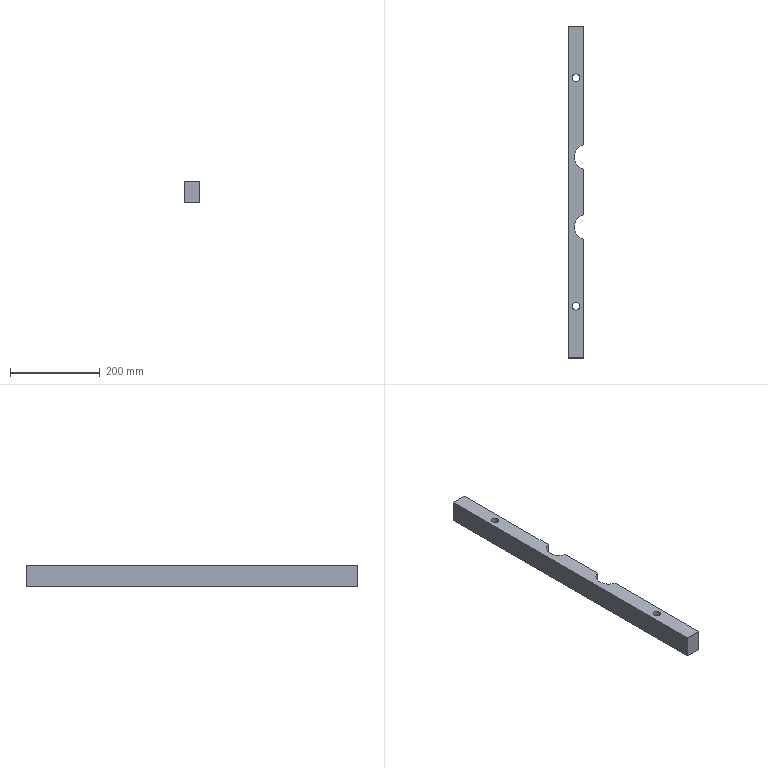Part | NX | features solid 2 | 1 solid | 12 faces | box 35 x 740 x 49 mm | volume 1163226 mm3 | plane 8 | cylinder 4 | commonest cylinder face diameters 17 x2 57 x2
STEP:
#1=CARTESIAN_POINT('',(868.,-370.,153.));
#2=VERTEX_POINT('',#1);
#3=CARTESIAN_POINT('',(868.,-370.,202.));
#4=VERTEX_POINT('',#3);
#5=CARTESIAN_POINT('',(868.,-370.,148.));
#6=DIRECTION('',(0.,0.,1.));
#7=VECTOR('',#6,1000.);
#8=LINE('',#5,#7);
#9=EDGE_CURVE('',#2,#4,#8,.T.);
#10=ORIENTED_EDGE('',*,*,#9,.F.);
#11=CARTESIAN_POINT('',(868.,-105.495,153.));
#12=VERTEX_POINT('',#11);
#13=CARTESIAN_POINT('',(868.,0.,153.));
#14=DIRECTION('',(0.,1.,0.));
#15=VECTOR('',#14,1000.);
#16=LINE('',#13,#15);
#17=EDGE_CURVE('',#2,#12,#16,.T.);
#18=ORIENTED_EDGE('',*,*,#17,.T.);
#19=CARTESIAN_POINT('',(868.,-105.495,202.));
#20=VERTEX_POINT('',#19);
#21=CARTESIAN_POINT('',(868.,-105.495,308.));
#22=DIRECTION('',(0.,0.,-1.));
#23=VECTOR('',#22,1000.);
#24=LINE('',#21,#23);
#25=EDGE_CURVE('',#12,#20,#24,.F.);
#26=ORIENTED_EDGE('',*,*,#25,.T.);
#27=CARTESIAN_POINT('',(868.,0.,202.));
#28=DIRECTION('',(0.,-1.,0.));
#29=VECTOR('',#28,1000.);
#30=LINE('',#27,#29);
#31=EDGE_CURVE('',#20,#4,#30,.T.);
#32=ORIENTED_EDGE('',*,*,#31,.T.);
#33=EDGE_LOOP('',(#10,#18,#26,#32));
#34=FACE_BOUND('',#33,.T.);
#35=CARTESIAN_POINT('',(868.,0.,148.));
#36=DIRECTION('',(1.,0.,0.));
#37=DIRECTION('',(0.,0.,-1.));
#38=AXIS2_PLACEMENT_3D('',#35,#36,#37);
#39=PLANE('',#38);
#40=ADVANCED_FACE('',(#34),#39,.T.);
#41=CARTESIAN_POINT('',(868.,-50.505,202.));
#42=VERTEX_POINT('',#41);
#43=CARTESIAN_POINT('',(868.,-50.505,153.));
#44=VERTEX_POINT('',#43);
#45=CARTESIAN_POINT('',(868.,-50.505,308.));
#46=DIRECTION('',(0.,0.,-1.));
#47=VECTOR('',#46,1000.);
#48=LINE('',#45,#47);
#49=EDGE_CURVE('',#42,#44,#48,.T.);
#50=ORIENTED_EDGE('',*,*,#49,.T.);
#51=CARTESIAN_POINT('',(868.,50.505,153.));
#52=VERTEX_POINT('',#51);
#53=CARTESIAN_POINT('',(868.,0.,153.));
#54=DIRECTION('',(0.,1.,0.));
#55=VECTOR('',#54,1000.);
#56=LINE('',#53,#55);
#57=EDGE_CURVE('',#44,#52,#56,.T.);
#58=ORIENTED_EDGE('',*,*,#57,.T.);
#59=CARTESIAN_POINT('',(868.,50.505,202.));
#60=VERTEX_POINT('',#59);
#61=CARTESIAN_POINT('',(868.,50.505,308.));
#62=DIRECTION('',(0.,0.,-1.));
#63=VECTOR('',#62,1000.);
#64=LINE('',#61,#63);
#65=EDGE_CURVE('',#52,#60,#64,.F.);
#66=ORIENTED_EDGE('',*,*,#65,.T.);
#67=CARTESIAN_POINT('',(868.,0.,202.));
#68=DIRECTION('',(0.,-1.,0.));
#69=VECTOR('',#68,1000.);
#70=LINE('',#67,#69);
#71=EDGE_CURVE('',#60,#42,#70,.T.);
#72=ORIENTED_EDGE('',*,*,#71,.T.);
#73=EDGE_LOOP('',(#50,#58,#66,#72));
#74=FACE_BOUND('',#73,.T.);
#75=CARTESIAN_POINT('',(868.,0.,148.));
#76=DIRECTION('',(1.,0.,0.));
#77=DIRECTION('',(0.,0.,-1.));
#78=AXIS2_PLACEMENT_3D('',#75,#76,#77);
#79=PLANE('',#78);
#80=ADVANCED_FACE('',(#74),#79,.T.);
#81=CARTESIAN_POINT('',(868.,105.495,202.));
#82=VERTEX_POINT('',#81);
#83=CARTESIAN_POINT('',(868.,105.495,153.));
#84=VERTEX_POINT('',#83);
#85=CARTESIAN_POINT('',(868.,105.495,308.));
#86=DIRECTION('',(0.,0.,-1.));
#87=VECTOR('',#86,1000.);
#88=LINE('',#85,#87);
#89=EDGE_CURVE('',#82,#84,#88,.T.);
#90=ORIENTED_EDGE('',*,*,#89,.T.);
#91=CARTESIAN_POINT('',(868.,370.,153.));
#92=VERTEX_POINT('',#91);
#93=CARTESIAN_POINT('',(868.,0.,153.));
#94=DIRECTION('',(0.,1.,0.));
#95=VECTOR('',#94,1000.);
#96=LINE('',#93,#95);
#97=EDGE_CURVE('',#84,#92,#96,.T.);
#98=ORIENTED_EDGE('',*,*,#97,.T.);
#99=CARTESIAN_POINT('',(868.,370.,202.));
#100=VERTEX_POINT('',#99);
#101=CARTESIAN_POINT('',(868.,370.,148.));
#102=DIRECTION('',(0.,0.,1.));
#103=VECTOR('',#102,1000.);
#104=LINE('',#101,#103);
#105=EDGE_CURVE('',#92,#100,#104,.T.);
#106=ORIENTED_EDGE('',*,*,#105,.T.);
#107=CARTESIAN_POINT('',(868.,0.,202.));
#108=DIRECTION('',(0.,-1.,0.));
#109=VECTOR('',#108,1000.);
#110=LINE('',#107,#109);
#111=EDGE_CURVE('',#100,#82,#110,.T.);
#112=ORIENTED_EDGE('',*,*,#111,.T.);
#113=EDGE_LOOP('',(#90,#98,#106,#112));
#114=FACE_BOUND('',#113,.T.);
#115=CARTESIAN_POINT('',(868.,0.,148.));
#116=DIRECTION('',(1.,0.,0.));
#117=DIRECTION('',(0.,0.,-1.));
#118=AXIS2_PLACEMENT_3D('',#115,#116,#117);
#119=PLANE('',#118);
#120=ADVANCED_FACE('',(#114),#119,.T.);
#121=CARTESIAN_POINT('',(842.,-255.,202.));
#122=VERTEX_POINT('',#121);
#123=CARTESIAN_POINT('',(850.5,-255.,202.));
#124=DIRECTION('',(0.,0.,1.));
#125=DIRECTION('',(-1.,0.,0.));
#126=AXIS2_PLACEMENT_3D('',#123,#124,#125);
#127=CIRCLE('',#126,8.5);
#128=EDGE_CURVE('',#122,#122,#127,.F.);
#129=ORIENTED_EDGE('',*,*,#128,.F.);
#130=EDGE_LOOP('',(#129));
#131=FACE_BOUND('',#130,.T.);
#132=CARTESIAN_POINT('',(842.,-255.,153.));
#133=VERTEX_POINT('',#132);
#134=CARTESIAN_POINT('',(850.5,-255.,153.));
#135=DIRECTION('',(0.,0.,-1.));
#136=DIRECTION('',(-1.,0.,0.));
#137=AXIS2_PLACEMENT_3D('',#134,#135,#136);
#138=CIRCLE('',#137,8.5);
#139=EDGE_CURVE('',#133,#133,#138,.F.);
#140=ORIENTED_EDGE('',*,*,#139,.F.);
#141=EDGE_LOOP('',(#140));
#142=FACE_BOUND('',#141,.T.);
#143=CARTESIAN_POINT('',(850.5,-255.,202.));
#144=DIRECTION('',(0.,0.,-1.));
#145=DIRECTION('',(-1.,0.,0.));
#146=AXIS2_PLACEMENT_3D('',#143,#144,#145);
#147=CYLINDRICAL_SURFACE('',#146,8.5);
#148=ADVANCED_FACE('',(#131,#142),#147,.F.);
#149=CARTESIAN_POINT('',(833.,370.,153.));
#150=VERTEX_POINT('',#149);
#151=CARTESIAN_POINT('',(833.,370.,202.));
#152=VERTEX_POINT('',#151);
#153=CARTESIAN_POINT('',(833.,370.,148.));
#154=DIRECTION('',(0.,0.,1.));
#155=VECTOR('',#154,1000.);
#156=LINE('',#153,#155);
#157=EDGE_CURVE('',#150,#152,#156,.T.);
#158=ORIENTED_EDGE('',*,*,#157,.F.);
#159=CARTESIAN_POINT('',(833.,-370.,153.));
#160=VERTEX_POINT('',#159);
#161=CARTESIAN_POINT('',(833.,0.,153.));
#162=DIRECTION('',(0.,-1.,0.));
#163=VECTOR('',#162,1000.);
#164=LINE('',#161,#163);
#165=EDGE_CURVE('',#150,#160,#164,.T.);
#166=ORIENTED_EDGE('',*,*,#165,.T.);
#167=CARTESIAN_POINT('',(833.,-370.,202.));
#168=VERTEX_POINT('',#167);
#169=CARTESIAN_POINT('',(833.,-370.,148.));
#170=DIRECTION('',(0.,0.,1.));
#171=VECTOR('',#170,1000.);
#172=LINE('',#169,#171);
#173=EDGE_CURVE('',#160,#168,#172,.T.);
#174=ORIENTED_EDGE('',*,*,#173,.T.);
#175=CARTESIAN_POINT('',(833.,0.,202.));
#176=DIRECTION('',(0.,1.,0.));
#177=VECTOR('',#176,1000.);
#178=LINE('',#175,#177);
#179=EDGE_CURVE('',#168,#152,#178,.T.);
#180=ORIENTED_EDGE('',*,*,#179,.T.);
#181=EDGE_LOOP('',(#158,#166,#174,#180));
#182=FACE_BOUND('',#181,.T.);
#183=CARTESIAN_POINT('',(833.,0.,148.));
#184=DIRECTION('',(-1.,0.,0.));
#185=DIRECTION('',(0.,0.,1.));
#186=AXIS2_PLACEMENT_3D('',#183,#184,#185);
#187=PLANE('',#186);
#188=ADVANCED_FACE('',(#182),#187,.T.);
#189=ORIENTED_EDGE('',*,*,#105,.F.);
#190=CARTESIAN_POINT('',(850.5,370.,153.));
#191=DIRECTION('',(-1.,0.,0.));
#192=VECTOR('',#191,1000.);
#193=LINE('',#190,#192);
#194=EDGE_CURVE('',#92,#150,#193,.T.);
#195=ORIENTED_EDGE('',*,*,#194,.T.);
#196=ORIENTED_EDGE('',*,*,#157,.T.);
#197=CARTESIAN_POINT('',(850.5,370.,202.));
#198=DIRECTION('',(1.,0.,0.));
#199=VECTOR('',#198,1000.);
#200=LINE('',#197,#199);
#201=EDGE_CURVE('',#152,#100,#200,.T.);
#202=ORIENTED_EDGE('',*,*,#201,.T.);
#203=EDGE_LOOP('',(#189,#195,#196,#202));
#204=FACE_BOUND('',#203,.T.);
#205=CARTESIAN_POINT('',(850.5,370.,148.));
#206=DIRECTION('',(0.,1.,0.));
#207=DIRECTION('',(0.,0.,1.));
#208=AXIS2_PLACEMENT_3D('',#205,#206,#207);
#209=PLANE('',#208);
#210=ADVANCED_FACE('',(#204),#209,.T.);
#211=ORIENTED_EDGE('',*,*,#173,.F.);
#212=CARTESIAN_POINT('',(850.5,-370.,153.));
#213=DIRECTION('',(1.,0.,0.));
#214=VECTOR('',#213,1000.);
#215=LINE('',#212,#214);
#216=EDGE_CURVE('',#160,#2,#215,.T.);
#217=ORIENTED_EDGE('',*,*,#216,.T.);
#218=ORIENTED_EDGE('',*,*,#9,.T.);
#219=CARTESIAN_POINT('',(850.5,-370.,202.));
#220=DIRECTION('',(-1.,0.,0.));
#221=VECTOR('',#220,1000.);
#222=LINE('',#219,#221);
#223=EDGE_CURVE('',#4,#168,#222,.T.);
#224=ORIENTED_EDGE('',*,*,#223,.T.);
#225=EDGE_LOOP('',(#211,#217,#218,#224));
#226=FACE_BOUND('',#225,.T.);
#227=CARTESIAN_POINT('',(850.5,-370.,148.));
#228=DIRECTION('',(0.,-1.,0.));
#229=DIRECTION('',(0.,0.,-1.));
#230=AXIS2_PLACEMENT_3D('',#227,#228,#229);
#231=PLANE('',#230);
#232=ADVANCED_FACE('',(#226),#231,.T.);
#233=CARTESIAN_POINT('',(842.,255.,202.));
#234=VERTEX_POINT('',#233);
#235=CARTESIAN_POINT('',(850.5,255.,202.));
#236=DIRECTION('',(0.,0.,-1.));
#237=DIRECTION('',(-1.,0.,0.));
#238=AXIS2_PLACEMENT_3D('',#235,#236,#237);
#239=CIRCLE('',#238,8.5);
#240=EDGE_CURVE('',#234,#234,#239,.T.);
#241=ORIENTED_EDGE('',*,*,#240,.F.);
#242=EDGE_LOOP('',(#241));
#243=FACE_BOUND('',#242,.T.);
#244=CARTESIAN_POINT('',(842.,255.,153.));
#245=VERTEX_POINT('',#244);
#246=CARTESIAN_POINT('',(850.5,255.,153.));
#247=DIRECTION('',(0.,0.,-1.));
#248=DIRECTION('',(-1.,0.,0.));
#249=AXIS2_PLACEMENT_3D('',#246,#247,#248);
#250=CIRCLE('',#249,8.5);
#251=EDGE_CURVE('',#245,#245,#250,.F.);
#252=ORIENTED_EDGE('',*,*,#251,.F.);
#253=EDGE_LOOP('',(#252));
#254=FACE_BOUND('',#253,.T.);
#255=CARTESIAN_POINT('',(850.5,255.,202.));
#256=DIRECTION('',(0.,0.,-1.));
#257=DIRECTION('',(-1.,0.,0.));
#258=AXIS2_PLACEMENT_3D('',#255,#256,#257);
#259=CYLINDRICAL_SURFACE('',#258,8.5);
#260=ADVANCED_FACE('',(#243,#254),#259,.F.);
#261=ORIENTED_EDGE('',*,*,#65,.F.);
#262=CARTESIAN_POINT('',(875.5,78.,153.));
#263=DIRECTION('',(0.,0.,-1.));
#264=DIRECTION('',(-1.,0.,0.));
#265=AXIS2_PLACEMENT_3D('',#262,#263,#264);
#266=CIRCLE('',#265,28.5);
#267=EDGE_CURVE('',#52,#84,#266,.T.);
#268=ORIENTED_EDGE('',*,*,#267,.T.);
#269=ORIENTED_EDGE('',*,*,#89,.F.);
#270=CARTESIAN_POINT('',(875.5,78.,202.));
#271=DIRECTION('',(0.,0.,1.));
#272=DIRECTION('',(1.,0.,0.));
#273=AXIS2_PLACEMENT_3D('',#270,#271,#272);
#274=CIRCLE('',#273,28.5);
#275=EDGE_CURVE('',#60,#82,#274,.F.);
#276=ORIENTED_EDGE('',*,*,#275,.F.);
#277=EDGE_LOOP('',(#261,#268,#269,#276));
#278=FACE_BOUND('',#277,.T.);
#279=CARTESIAN_POINT('',(875.5,78.,308.));
#280=DIRECTION('',(0.,0.,-1.));
#281=DIRECTION('',(-1.,0.,0.));
#282=AXIS2_PLACEMENT_3D('',#279,#280,#281);
#283=CYLINDRICAL_SURFACE('',#282,28.5);
#284=ADVANCED_FACE('',(#278),#283,.F.);
#285=ORIENTED_EDGE('',*,*,#25,.F.);
#286=CARTESIAN_POINT('',(875.5,-78.,153.));
#287=DIRECTION('',(0.,0.,-1.));
#288=DIRECTION('',(-1.,0.,0.));
#289=AXIS2_PLACEMENT_3D('',#286,#287,#288);
#290=CIRCLE('',#289,28.5);
#291=EDGE_CURVE('',#12,#44,#290,.T.);
#292=ORIENTED_EDGE('',*,*,#291,.T.);
#293=ORIENTED_EDGE('',*,*,#49,.F.);
#294=CARTESIAN_POINT('',(875.5,-78.,202.));
#295=DIRECTION('',(0.,0.,1.));
#296=DIRECTION('',(1.,0.,0.));
#297=AXIS2_PLACEMENT_3D('',#294,#295,#296);
#298=CIRCLE('',#297,28.5);
#299=EDGE_CURVE('',#20,#42,#298,.F.);
#300=ORIENTED_EDGE('',*,*,#299,.F.);
#301=EDGE_LOOP('',(#285,#292,#293,#300));
#302=FACE_BOUND('',#301,.T.);
#303=CARTESIAN_POINT('',(875.5,-78.,308.));
#304=DIRECTION('',(0.,0.,-1.));
#305=DIRECTION('',(-1.,0.,0.));
#306=AXIS2_PLACEMENT_3D('',#303,#304,#305);
#307=CYLINDRICAL_SURFACE('',#306,28.5);
#308=ADVANCED_FACE('',(#302),#307,.F.);
#309=ORIENTED_EDGE('',*,*,#128,.T.);
#310=EDGE_LOOP('',(#309));
#311=FACE_BOUND('',#310,.T.);
#312=ORIENTED_EDGE('',*,*,#240,.T.);
#313=EDGE_LOOP('',(#312));
#314=FACE_BOUND('',#313,.T.);
#315=ORIENTED_EDGE('',*,*,#31,.F.);
#316=ORIENTED_EDGE('',*,*,#299,.T.);
#317=ORIENTED_EDGE('',*,*,#71,.F.);
#318=ORIENTED_EDGE('',*,*,#275,.T.);
#319=ORIENTED_EDGE('',*,*,#111,.F.);
#320=ORIENTED_EDGE('',*,*,#201,.F.);
#321=ORIENTED_EDGE('',*,*,#179,.F.);
#322=ORIENTED_EDGE('',*,*,#223,.F.);
#323=EDGE_LOOP('',(#315,#316,#317,#318,#319,#320,#321,#322));
#324=FACE_BOUND('',#323,.T.);
#325=CARTESIAN_POINT('',(850.5,0.,202.));
#326=DIRECTION('',(0.,0.,1.));
#327=DIRECTION('',(1.,0.,0.));
#328=AXIS2_PLACEMENT_3D('',#325,#326,#327);
#329=PLANE('',#328);
#330=ADVANCED_FACE('',(#311,#314,#324),#329,.T.);
#331=ORIENTED_EDGE('',*,*,#251,.T.);
#332=EDGE_LOOP('',(#331));
#333=FACE_BOUND('',#332,.T.);
#334=ORIENTED_EDGE('',*,*,#194,.F.);
#335=ORIENTED_EDGE('',*,*,#97,.F.);
#336=ORIENTED_EDGE('',*,*,#267,.F.);
#337=ORIENTED_EDGE('',*,*,#57,.F.);
#338=ORIENTED_EDGE('',*,*,#291,.F.);
#339=ORIENTED_EDGE('',*,*,#17,.F.);
#340=ORIENTED_EDGE('',*,*,#216,.F.);
#341=ORIENTED_EDGE('',*,*,#165,.F.);
#342=EDGE_LOOP('',(#334,#335,#336,#337,#338,#339,#340,#341));
#343=FACE_BOUND('',#342,.T.);
#344=ORIENTED_EDGE('',*,*,#139,.T.);
#345=EDGE_LOOP('',(#344));
#346=FACE_BOUND('',#345,.T.);
#347=CARTESIAN_POINT('',(835.5,0.,153.));
#348=DIRECTION('',(0.,0.,-1.));
#349=DIRECTION('',(-1.,0.,0.));
#350=AXIS2_PLACEMENT_3D('',#347,#348,#349);
#351=PLANE('',#350);
#352=ADVANCED_FACE('',(#333,#343,#346),#351,.T.);
#353=CLOSED_SHELL('',(#40,#80,#120,#148,#188,#210,#232,#260,#284,#308,#330,#352));
#354=MANIFOLD_SOLID_BREP('',#353);
#355=(LENGTH_UNIT()NAMED_UNIT(*)SI_UNIT(.MILLI.,.METRE.));
#356=UNCERTAINTY_MEASURE_WITH_UNIT(LENGTH_MEASURE(0.00001),#355,'','');
#357=(NAMED_UNIT(*)PLANE_ANGLE_UNIT()SI_UNIT($,.RADIAN.));
#358=(NAMED_UNIT(*)SI_UNIT($,.STERADIAN.)SOLID_ANGLE_UNIT());
#359=(GEOMETRIC_REPRESENTATION_CONTEXT(3)GLOBAL_UNCERTAINTY_ASSIGNED_CONTEXT((#356))GLOBAL_UNIT_ASSIGNED_CONTEXT((#355,#357,#358))REPRESENTATION_CONTEXT('',''));
#360=ADVANCED_BREP_SHAPE_REPRESENTATION('',(#354),#359);